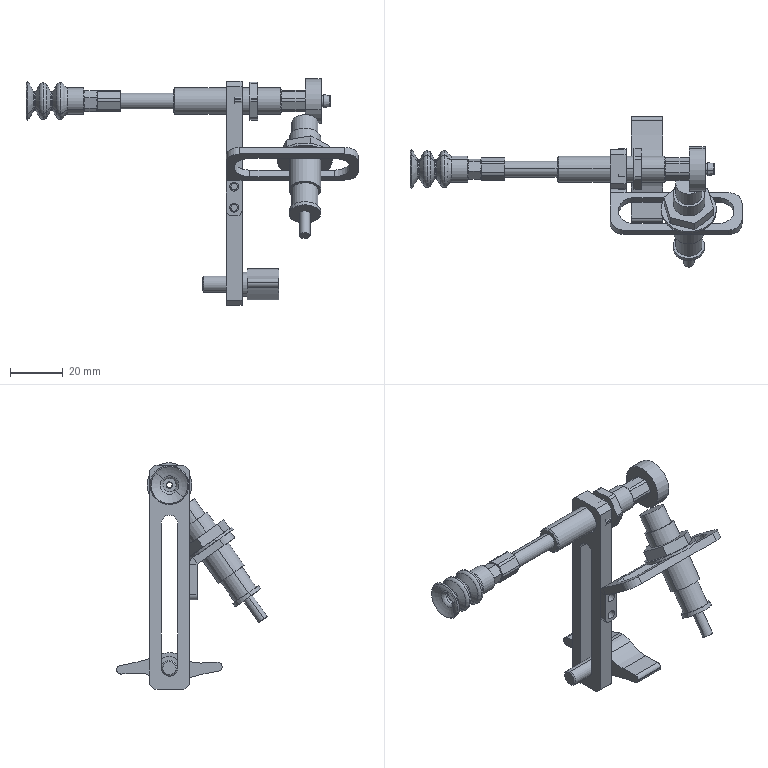Part | SolidWorks | 14 solids | 373 faces | box 126 x 57.116 x 86 mm | volume 21560 mm3 | cylinder 137 | plane 132 | cone 58 | torus 44 | sphere 2 | commonest cylinder face diameters 15.5 x16 8.7 x12 10 x11 12 x11 5 x10 4 x8